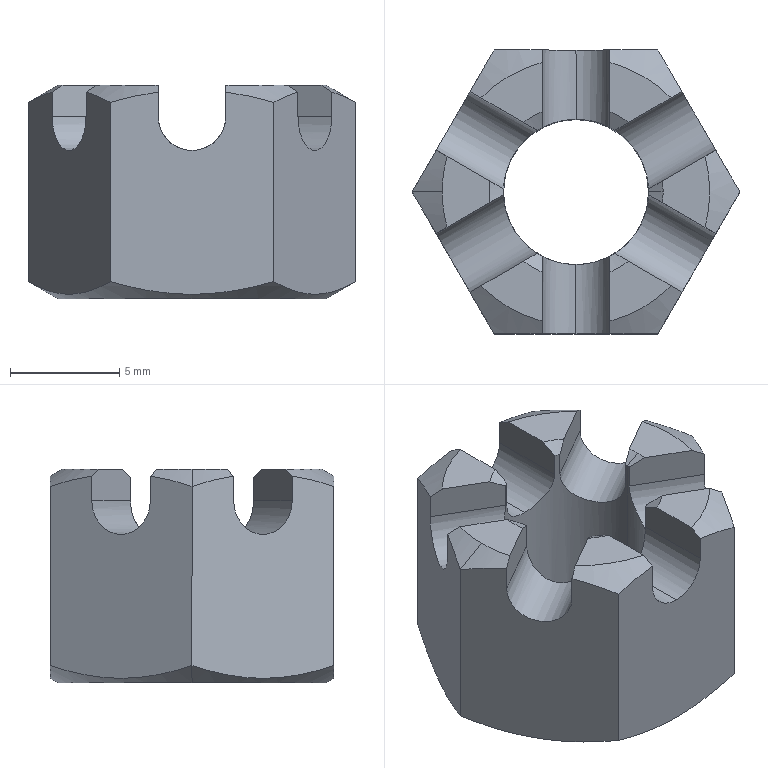Part | STEP file | hex slotted and castle nuts 1-grade ab gb_GB_FASTENER_NUT_SNNAB1 M8 YB-N | 1 solid | 53 faces | box 15.011 x 13 x 9.8 mm | volume 915.149 mm3 | plane 25 | cone 18 | cylinder 10 | commonest cylinder face diameters 3.1 x8 6.647 x2